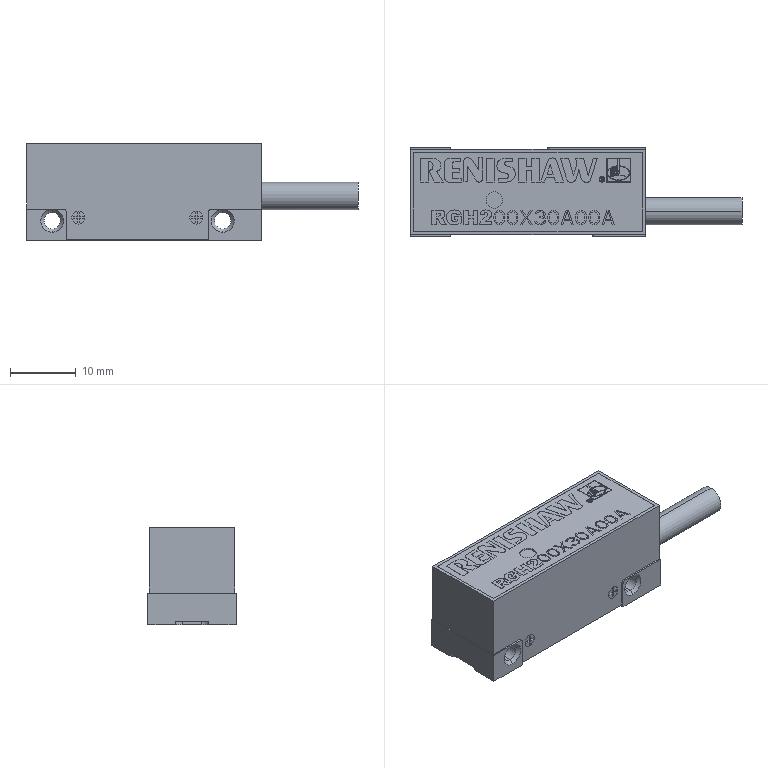Part | NX | features BREP 1 | 1 solid | 764 faces | box 50.65 x 13.5 x 14.8 mm | volume 6947 mm3 | plane 612 | spline 82 | cylinder 62 | cone 8 | commonest cylinder face diameters 2.5 x12 2 x6 1 x4 4.3 x3 0.376 x2 0.38 x2